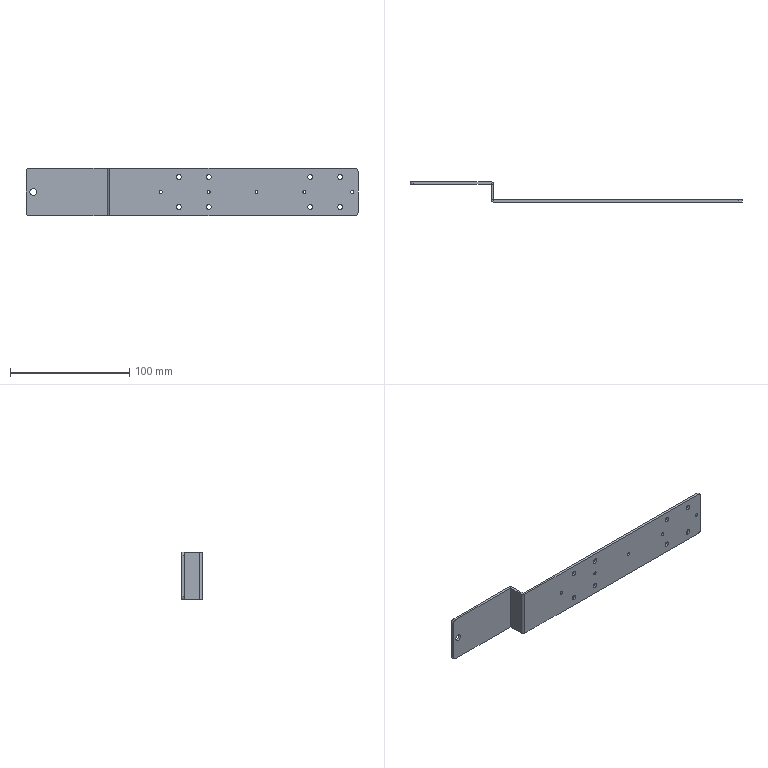Part | SolidWorks | features EdgeFlange 2, HoleWzd 2, Fillet 1, FlatPattern 1, ICE 1, LPattern 1, SMBaseFlange 1, SheetMetal 1 | 1 solid | 54 faces | box 278 x 17 x 40 mm | volume 23031 mm3 | cylinder 36 | plane 18 | commonest cylinder face diameters 4.2 x18 2.5 x10 6 x4 0.2 x2 5.5 x2